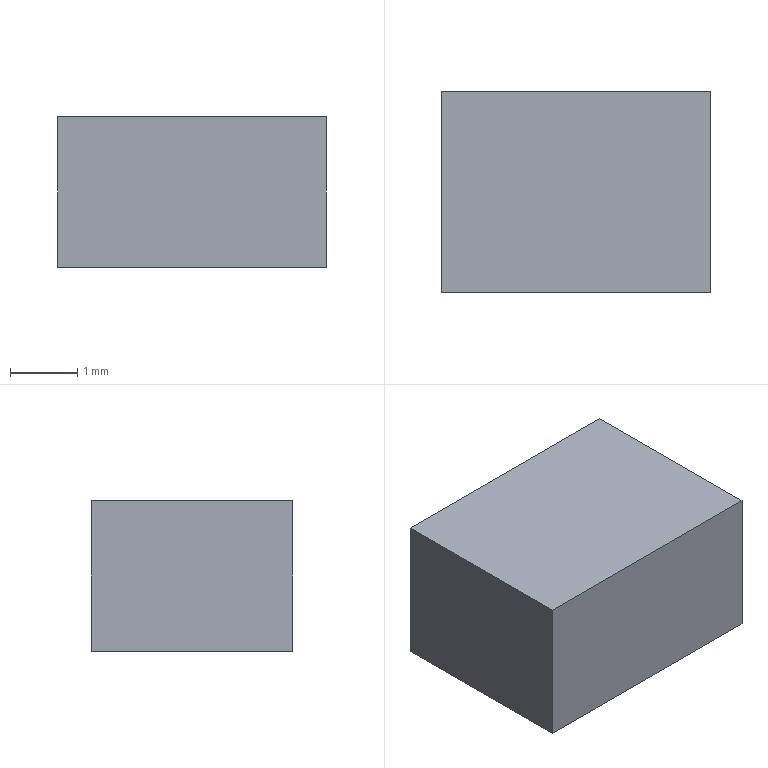Part | Creo | 1 solid | 6 faces | box 4 x 3 x 2.25 mm | volume 27 mm3 | plane 6
STEP:
#1=CARTESIAN_POINT('',(0.,0.,0.));
#2=DIRECTION('',(0.,0.,1.));
#3=DIRECTION('',(1.,0.,0.));
#4=AXIS2_PLACEMENT_3D('',#1,#2,#3);
#5=CARTESIAN_POINT('',(3.25,-1.5,0.));
#6=VERTEX_POINT('',#5);
#7=CARTESIAN_POINT('',(-0.75,-1.5,0.));
#8=VERTEX_POINT('',#7);
#9=CARTESIAN_POINT('',(3.25,-1.5,0.));
#10=DIRECTION('',(-1.,0.,0.));
#11=VECTOR('',#10,4.);
#12=LINE('',#9,#11);
#13=EDGE_CURVE('',#6,#8,#12,.T.);
#14=ORIENTED_EDGE('',*,*,#13,.F.);
#15=CARTESIAN_POINT('',(3.25,1.5,0.));
#16=VERTEX_POINT('',#15);
#17=CARTESIAN_POINT('',(3.25,1.5,0.));
#18=DIRECTION('',(0.,-1.,0.));
#19=VECTOR('',#18,3.);
#20=LINE('',#17,#19);
#21=EDGE_CURVE('',#16,#6,#20,.T.);
#22=ORIENTED_EDGE('',*,*,#21,.F.);
#23=CARTESIAN_POINT('',(-0.75,1.5,0.));
#24=VERTEX_POINT('',#23);
#25=CARTESIAN_POINT('',(-0.75,1.5,0.));
#26=DIRECTION('',(1.,0.,0.));
#27=VECTOR('',#26,4.);
#28=LINE('',#25,#27);
#29=EDGE_CURVE('',#24,#16,#28,.T.);
#30=ORIENTED_EDGE('',*,*,#29,.F.);
#31=CARTESIAN_POINT('',(-0.75,-1.5,0.));
#32=DIRECTION('',(0.,1.,0.));
#33=VECTOR('',#32,3.);
#34=LINE('',#31,#33);
#35=EDGE_CURVE('',#8,#24,#34,.T.);
#36=ORIENTED_EDGE('',*,*,#35,.F.);
#37=EDGE_LOOP('',(#14,#22,#30,#36));
#38=FACE_OUTER_BOUND('',#37,.F.);
#39=CARTESIAN_POINT('',(0.,0.,0.));
#40=DIRECTION('',(0.,0.,1.));
#41=DIRECTION('',(1.,0.,0.));
#42=AXIS2_PLACEMENT_3D('',#39,#40,#41);
#43=PLANE('',#42);
#44=ADVANCED_FACE('',(#38),#43,.F.);
#45=ORIENTED_EDGE('',*,*,#13,.T.);
#46=CARTESIAN_POINT('',(-0.75,-1.5,2.25));
#47=VERTEX_POINT('',#46);
#48=CARTESIAN_POINT('',(-0.75,-1.5,2.25));
#49=DIRECTION('',(0.,0.,-1.));
#50=VECTOR('',#49,2.25);
#51=LINE('',#48,#50);
#52=EDGE_CURVE('',#47,#8,#51,.T.);
#53=ORIENTED_EDGE('',*,*,#52,.F.);
#54=CARTESIAN_POINT('',(3.25,-1.5,2.25));
#55=VERTEX_POINT('',#54);
#56=CARTESIAN_POINT('',(3.25,-1.5,2.25));
#57=DIRECTION('',(-1.,0.,0.));
#58=VECTOR('',#57,4.);
#59=LINE('',#56,#58);
#60=EDGE_CURVE('',#55,#47,#59,.T.);
#61=ORIENTED_EDGE('',*,*,#60,.F.);
#62=CARTESIAN_POINT('',(3.25,-1.5,2.25));
#63=DIRECTION('',(0.,0.,-1.));
#64=VECTOR('',#63,2.25);
#65=LINE('',#62,#64);
#66=EDGE_CURVE('',#55,#6,#65,.T.);
#67=ORIENTED_EDGE('',*,*,#66,.T.);
#68=EDGE_LOOP('',(#45,#53,#61,#67));
#69=FACE_OUTER_BOUND('',#68,.F.);
#70=CARTESIAN_POINT('',(-0.75,-1.5,0.));
#71=DIRECTION('',(0.,-1.,0.));
#72=DIRECTION('',(1.,0.,0.));
#73=AXIS2_PLACEMENT_3D('',#70,#71,#72);
#74=PLANE('',#73);
#75=ADVANCED_FACE('',(#69),#74,.T.);
#76=ORIENTED_EDGE('',*,*,#35,.T.);
#77=CARTESIAN_POINT('',(-0.75,1.5,2.25));
#78=VERTEX_POINT('',#77);
#79=CARTESIAN_POINT('',(-0.75,1.5,2.25));
#80=DIRECTION('',(0.,0.,-1.));
#81=VECTOR('',#80,2.25);
#82=LINE('',#79,#81);
#83=EDGE_CURVE('',#78,#24,#82,.T.);
#84=ORIENTED_EDGE('',*,*,#83,.F.);
#85=CARTESIAN_POINT('',(-0.75,-1.5,2.25));
#86=DIRECTION('',(0.,1.,0.));
#87=VECTOR('',#86,3.);
#88=LINE('',#85,#87);
#89=EDGE_CURVE('',#47,#78,#88,.T.);
#90=ORIENTED_EDGE('',*,*,#89,.F.);
#91=ORIENTED_EDGE('',*,*,#52,.T.);
#92=EDGE_LOOP('',(#76,#84,#90,#91));
#93=FACE_OUTER_BOUND('',#92,.F.);
#94=CARTESIAN_POINT('',(-0.75,1.5,0.));
#95=DIRECTION('',(-1.,0.,0.));
#96=DIRECTION('',(0.,-1.,0.));
#97=AXIS2_PLACEMENT_3D('',#94,#95,#96);
#98=PLANE('',#97);
#99=ADVANCED_FACE('',(#93),#98,.T.);
#100=ORIENTED_EDGE('',*,*,#29,.T.);
#101=CARTESIAN_POINT('',(3.25,1.5,2.25));
#102=VERTEX_POINT('',#101);
#103=CARTESIAN_POINT('',(3.25,1.5,2.25));
#104=DIRECTION('',(0.,0.,-1.));
#105=VECTOR('',#104,2.25);
#106=LINE('',#103,#105);
#107=EDGE_CURVE('',#102,#16,#106,.T.);
#108=ORIENTED_EDGE('',*,*,#107,.F.);
#109=CARTESIAN_POINT('',(-0.75,1.5,2.25));
#110=DIRECTION('',(1.,0.,0.));
#111=VECTOR('',#110,4.);
#112=LINE('',#109,#111);
#113=EDGE_CURVE('',#78,#102,#112,.T.);
#114=ORIENTED_EDGE('',*,*,#113,.F.);
#115=ORIENTED_EDGE('',*,*,#83,.T.);
#116=EDGE_LOOP('',(#100,#108,#114,#115));
#117=FACE_OUTER_BOUND('',#116,.F.);
#118=CARTESIAN_POINT('',(3.25,1.5,0.));
#119=DIRECTION('',(0.,1.,0.));
#120=DIRECTION('',(-1.,0.,0.));
#121=AXIS2_PLACEMENT_3D('',#118,#119,#120);
#122=PLANE('',#121);
#123=ADVANCED_FACE('',(#117),#122,.T.);
#124=ORIENTED_EDGE('',*,*,#21,.T.);
#125=ORIENTED_EDGE('',*,*,#66,.F.);
#126=CARTESIAN_POINT('',(3.25,1.5,2.25));
#127=DIRECTION('',(0.,-1.,0.));
#128=VECTOR('',#127,3.);
#129=LINE('',#126,#128);
#130=EDGE_CURVE('',#102,#55,#129,.T.);
#131=ORIENTED_EDGE('',*,*,#130,.F.);
#132=ORIENTED_EDGE('',*,*,#107,.T.);
#133=EDGE_LOOP('',(#124,#125,#131,#132));
#134=FACE_OUTER_BOUND('',#133,.F.);
#135=CARTESIAN_POINT('',(3.25,-1.5,0.));
#136=DIRECTION('',(1.,0.,0.));
#137=DIRECTION('',(0.,1.,0.));
#138=AXIS2_PLACEMENT_3D('',#135,#136,#137);
#139=PLANE('',#138);
#140=ADVANCED_FACE('',(#134),#139,.T.);
#141=ORIENTED_EDGE('',*,*,#60,.T.);
#142=ORIENTED_EDGE('',*,*,#89,.T.);
#143=ORIENTED_EDGE('',*,*,#113,.T.);
#144=ORIENTED_EDGE('',*,*,#130,.T.);
#145=EDGE_LOOP('',(#141,#142,#143,#144));
#146=FACE_OUTER_BOUND('',#145,.F.);
#147=CARTESIAN_POINT('',(0.,0.,2.25));
#148=DIRECTION('',(0.,0.,1.));
#149=DIRECTION('',(1.,0.,0.));
#150=AXIS2_PLACEMENT_3D('',#147,#148,#149);
#151=PLANE('',#150);
#152=ADVANCED_FACE('',(#146),#151,.T.);
#153=CLOSED_SHELL('',(#44,#75,#99,#123,#140,#152));
#154=MANIFOLD_SOLID_BREP('',#153);
#155=(LENGTH_UNIT()NAMED_UNIT(*)SI_UNIT(.MILLI.,.METRE.));
#156=UNCERTAINTY_MEASURE_WITH_UNIT(LENGTH_MEASURE(0.0005483),#155,'','');
#157=(NAMED_UNIT(*)PLANE_ANGLE_UNIT()SI_UNIT($,.RADIAN.));
#158=PLANE_ANGLE_MEASURE_WITH_UNIT(PLANE_ANGLE_MEASURE(0.01745),#157);
#159=(CONVERSION_BASED_UNIT('DEGREE',#158)NAMED_UNIT(*)PLANE_ANGLE_UNIT());
#160=(NAMED_UNIT(*)SI_UNIT($,.STERADIAN.)SOLID_ANGLE_UNIT());
#161=(GEOMETRIC_REPRESENTATION_CONTEXT(3)GLOBAL_UNCERTAINTY_ASSIGNED_CONTEXT((#156))GLOBAL_UNIT_ASSIGNED_CONTEXT((#155,#159,#160))REPRESENTATION_CONTEXT('',''));
#162=ADVANCED_BREP_SHAPE_REPRESENTATION('',(#4,#154),#161);